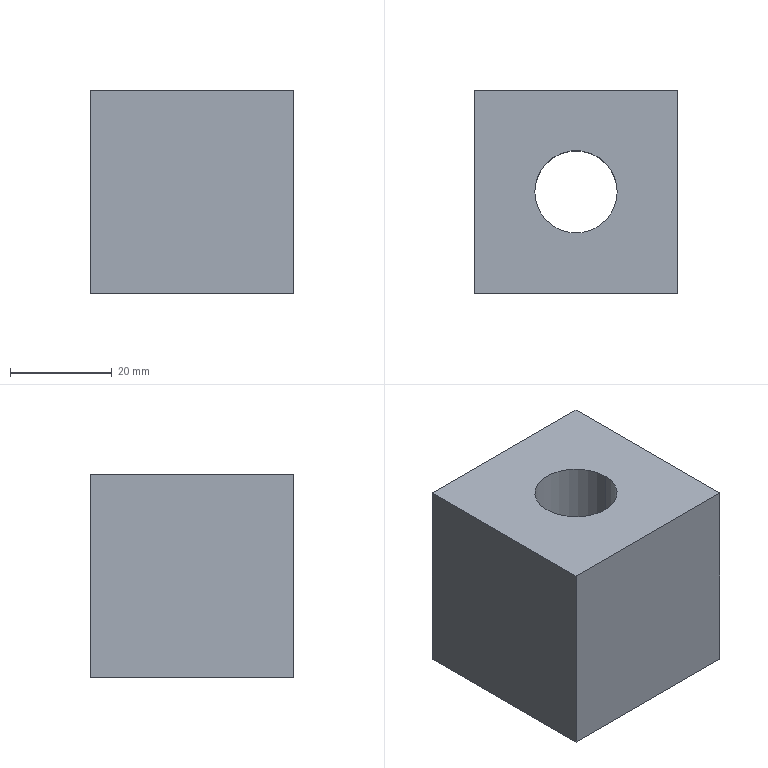Part | SolidWorks | features Extrusion 1, ICE 1 | 1 solid | 8 faces | box 40 x 40 x 40 mm | volume 55755 mm3 | plane 6 | cylinder 2 | commonest cylinder face diameters 16.2 x2
STEP:
#1=CARTESIAN_POINT('',(-8.1,0.,-20.));
#2=VERTEX_POINT('',#1);
#3=CARTESIAN_POINT('',(8.1,0.,-20.));
#4=VERTEX_POINT('',#3);
#5=CARTESIAN_POINT('',(0.,0.,-20.));
#6=DIRECTION('',(0.,0.,1.));
#7=DIRECTION('',(1.,0.,0.));
#8=AXIS2_PLACEMENT_3D('',#5,#6,#7);
#9=CIRCLE('',#8,8.1);
#10=EDGE_CURVE('',#2,#4,#9,.T.);
#11=ORIENTED_EDGE('',*,*,#10,.F.);
#12=CARTESIAN_POINT('',(-8.1,0.,20.));
#13=VERTEX_POINT('',#12);
#14=CARTESIAN_POINT('',(-8.1,0.,-40.));
#15=DIRECTION('',(0.,0.,1.));
#16=VECTOR('',#15,1000.);
#17=LINE('',#14,#16);
#18=EDGE_CURVE('',#2,#13,#17,.T.);
#19=ORIENTED_EDGE('',*,*,#18,.T.);
#20=CARTESIAN_POINT('',(8.1,0.,20.));
#21=VERTEX_POINT('',#20);
#22=CARTESIAN_POINT('',(0.,0.,20.));
#23=DIRECTION('',(0.,0.,1.));
#24=DIRECTION('',(1.,0.,0.));
#25=AXIS2_PLACEMENT_3D('',#22,#23,#24);
#26=CIRCLE('',#25,8.1);
#27=EDGE_CURVE('',#13,#21,#26,.T.);
#28=ORIENTED_EDGE('',*,*,#27,.T.);
#29=CARTESIAN_POINT('',(8.1,0.,-40.));
#30=DIRECTION('',(0.,0.,1.));
#31=VECTOR('',#30,1000.);
#32=LINE('',#29,#31);
#33=EDGE_CURVE('',#4,#21,#32,.T.);
#34=ORIENTED_EDGE('',*,*,#33,.F.);
#35=EDGE_LOOP('',(#11,#19,#28,#34));
#36=FACE_OUTER_BOUND('',#35,.T.);
#37=CARTESIAN_POINT('',(0.,0.,-40.));
#38=DIRECTION('',(0.,0.,1.));
#39=DIRECTION('',(1.,0.,0.));
#40=AXIS2_PLACEMENT_3D('',#37,#38,#39);
#41=CYLINDRICAL_SURFACE('',#40,8.1);
#42=ADVANCED_FACE('',(#36),#41,.F.);
#43=CARTESIAN_POINT('',(-20.,20.,20.));
#44=VERTEX_POINT('',#43);
#45=CARTESIAN_POINT('',(-20.,-20.,20.));
#46=VERTEX_POINT('',#45);
#47=CARTESIAN_POINT('',(-20.,20.,20.));
#48=DIRECTION('',(0.,-1.,0.));
#49=VECTOR('',#48,1000.);
#50=LINE('',#47,#49);
#51=EDGE_CURVE('',#44,#46,#50,.T.);
#52=ORIENTED_EDGE('',*,*,#51,.F.);
#53=CARTESIAN_POINT('',(-20.,20.,-20.));
#54=VERTEX_POINT('',#53);
#55=CARTESIAN_POINT('',(-20.,20.,-20.));
#56=DIRECTION('',(0.,0.,1.));
#57=VECTOR('',#56,1000.);
#58=LINE('',#55,#57);
#59=EDGE_CURVE('',#54,#44,#58,.T.);
#60=ORIENTED_EDGE('',*,*,#59,.F.);
#61=CARTESIAN_POINT('',(-20.,-20.,-20.));
#62=VERTEX_POINT('',#61);
#63=CARTESIAN_POINT('',(-20.,20.,-20.));
#64=DIRECTION('',(0.,-1.,0.));
#65=VECTOR('',#64,1000.);
#66=LINE('',#63,#65);
#67=EDGE_CURVE('',#54,#62,#66,.T.);
#68=ORIENTED_EDGE('',*,*,#67,.T.);
#69=CARTESIAN_POINT('',(-20.,-20.,-20.));
#70=DIRECTION('',(0.,0.,1.));
#71=VECTOR('',#70,1000.);
#72=LINE('',#69,#71);
#73=EDGE_CURVE('',#62,#46,#72,.T.);
#74=ORIENTED_EDGE('',*,*,#73,.T.);
#75=EDGE_LOOP('',(#52,#60,#68,#74));
#76=FACE_OUTER_BOUND('',#75,.T.);
#77=CARTESIAN_POINT('',(-20.,20.,-20.));
#78=DIRECTION('',(-1.,0.,0.));
#79=DIRECTION('',(0.,0.,1.));
#80=AXIS2_PLACEMENT_3D('',#77,#78,#79);
#81=PLANE('',#80);
#82=ADVANCED_FACE('',(#76),#81,.T.);
#83=CARTESIAN_POINT('',(20.,20.,20.));
#84=VERTEX_POINT('',#83);
#85=CARTESIAN_POINT('',(20.,20.,20.));
#86=DIRECTION('',(-1.,0.,0.));
#87=VECTOR('',#86,1000.);
#88=LINE('',#85,#87);
#89=EDGE_CURVE('',#84,#44,#88,.T.);
#90=ORIENTED_EDGE('',*,*,#89,.F.);
#91=CARTESIAN_POINT('',(20.,20.,-20.));
#92=VERTEX_POINT('',#91);
#93=CARTESIAN_POINT('',(20.,20.,-20.));
#94=DIRECTION('',(0.,0.,1.));
#95=VECTOR('',#94,1000.);
#96=LINE('',#93,#95);
#97=EDGE_CURVE('',#92,#84,#96,.T.);
#98=ORIENTED_EDGE('',*,*,#97,.F.);
#99=CARTESIAN_POINT('',(20.,20.,-20.));
#100=DIRECTION('',(-1.,0.,0.));
#101=VECTOR('',#100,1000.);
#102=LINE('',#99,#101);
#103=EDGE_CURVE('',#92,#54,#102,.T.);
#104=ORIENTED_EDGE('',*,*,#103,.T.);
#105=ORIENTED_EDGE('',*,*,#59,.T.);
#106=EDGE_LOOP('',(#90,#98,#104,#105));
#107=FACE_OUTER_BOUND('',#106,.T.);
#108=CARTESIAN_POINT('',(20.,20.,-20.));
#109=DIRECTION('',(0.,1.,0.));
#110=DIRECTION('',(0.,0.,1.));
#111=AXIS2_PLACEMENT_3D('',#108,#109,#110);
#112=PLANE('',#111);
#113=ADVANCED_FACE('',(#107),#112,.T.);
#114=CARTESIAN_POINT('',(20.,-20.,20.));
#115=VERTEX_POINT('',#114);
#116=CARTESIAN_POINT('',(20.,-20.,20.));
#117=DIRECTION('',(0.,1.,0.));
#118=VECTOR('',#117,1000.);
#119=LINE('',#116,#118);
#120=EDGE_CURVE('',#115,#84,#119,.T.);
#121=ORIENTED_EDGE('',*,*,#120,.F.);
#122=CARTESIAN_POINT('',(20.,-20.,-20.));
#123=VERTEX_POINT('',#122);
#124=CARTESIAN_POINT('',(20.,-20.,-20.));
#125=DIRECTION('',(0.,0.,1.));
#126=VECTOR('',#125,1000.);
#127=LINE('',#124,#126);
#128=EDGE_CURVE('',#123,#115,#127,.T.);
#129=ORIENTED_EDGE('',*,*,#128,.F.);
#130=CARTESIAN_POINT('',(20.,-20.,-20.));
#131=DIRECTION('',(0.,1.,0.));
#132=VECTOR('',#131,1000.);
#133=LINE('',#130,#132);
#134=EDGE_CURVE('',#123,#92,#133,.T.);
#135=ORIENTED_EDGE('',*,*,#134,.T.);
#136=ORIENTED_EDGE('',*,*,#97,.T.);
#137=EDGE_LOOP('',(#121,#129,#135,#136));
#138=FACE_OUTER_BOUND('',#137,.T.);
#139=CARTESIAN_POINT('',(20.,-20.,-20.));
#140=DIRECTION('',(1.,0.,0.));
#141=DIRECTION('',(0.,0.,-1.));
#142=AXIS2_PLACEMENT_3D('',#139,#140,#141);
#143=PLANE('',#142);
#144=ADVANCED_FACE('',(#138),#143,.T.);
#145=CARTESIAN_POINT('',(-20.,-20.,20.));
#146=DIRECTION('',(1.,0.,0.));
#147=VECTOR('',#146,1000.);
#148=LINE('',#145,#147);
#149=EDGE_CURVE('',#46,#115,#148,.T.);
#150=ORIENTED_EDGE('',*,*,#149,.F.);
#151=ORIENTED_EDGE('',*,*,#73,.F.);
#152=CARTESIAN_POINT('',(-20.,-20.,-20.));
#153=DIRECTION('',(1.,0.,0.));
#154=VECTOR('',#153,1000.);
#155=LINE('',#152,#154);
#156=EDGE_CURVE('',#62,#123,#155,.T.);
#157=ORIENTED_EDGE('',*,*,#156,.T.);
#158=ORIENTED_EDGE('',*,*,#128,.T.);
#159=EDGE_LOOP('',(#150,#151,#157,#158));
#160=FACE_OUTER_BOUND('',#159,.T.);
#161=CARTESIAN_POINT('',(-20.,-20.,-20.));
#162=DIRECTION('',(0.,-1.,0.));
#163=DIRECTION('',(0.,0.,-1.));
#164=AXIS2_PLACEMENT_3D('',#161,#162,#163);
#165=PLANE('',#164);
#166=ADVANCED_FACE('',(#160),#165,.T.);
#167=CARTESIAN_POINT('',(0.,0.,-20.));
#168=DIRECTION('',(0.,0.,1.));
#169=DIRECTION('',(1.,0.,0.));
#170=AXIS2_PLACEMENT_3D('',#167,#168,#169);
#171=CIRCLE('',#170,8.1);
#172=EDGE_CURVE('',#4,#2,#171,.T.);
#173=ORIENTED_EDGE('',*,*,#172,.T.);
#174=ORIENTED_EDGE('',*,*,#10,.T.);
#175=EDGE_LOOP('',(#173,#174));
#176=FACE_BOUND('',#175,.T.);
#177=ORIENTED_EDGE('',*,*,#67,.F.);
#178=ORIENTED_EDGE('',*,*,#103,.F.);
#179=ORIENTED_EDGE('',*,*,#134,.F.);
#180=ORIENTED_EDGE('',*,*,#156,.F.);
#181=EDGE_LOOP('',(#177,#178,#179,#180));
#182=FACE_OUTER_BOUND('',#181,.T.);
#183=CARTESIAN_POINT('',(0.,0.,-20.));
#184=DIRECTION('',(0.,0.,1.));
#185=DIRECTION('',(1.,0.,0.));
#186=AXIS2_PLACEMENT_3D('',#183,#184,#185);
#187=PLANE('',#186);
#188=ADVANCED_FACE('',(#176,#182),#187,.F.);
#189=CARTESIAN_POINT('',(0.,0.,20.));
#190=DIRECTION('',(0.,0.,1.));
#191=DIRECTION('',(1.,0.,0.));
#192=AXIS2_PLACEMENT_3D('',#189,#190,#191);
#193=CIRCLE('',#192,8.1);
#194=EDGE_CURVE('',#21,#13,#193,.T.);
#195=ORIENTED_EDGE('',*,*,#194,.F.);
#196=ORIENTED_EDGE('',*,*,#27,.F.);
#197=EDGE_LOOP('',(#195,#196));
#198=FACE_BOUND('',#197,.T.);
#199=ORIENTED_EDGE('',*,*,#51,.T.);
#200=ORIENTED_EDGE('',*,*,#149,.T.);
#201=ORIENTED_EDGE('',*,*,#120,.T.);
#202=ORIENTED_EDGE('',*,*,#89,.T.);
#203=EDGE_LOOP('',(#199,#200,#201,#202));
#204=FACE_OUTER_BOUND('',#203,.T.);
#205=CARTESIAN_POINT('',(0.,0.,20.));
#206=DIRECTION('',(0.,0.,1.));
#207=DIRECTION('',(1.,0.,0.));
#208=AXIS2_PLACEMENT_3D('',#205,#206,#207);
#209=PLANE('',#208);
#210=ADVANCED_FACE('',(#198,#204),#209,.T.);
#211=ORIENTED_EDGE('',*,*,#18,.F.);
#212=ORIENTED_EDGE('',*,*,#172,.F.);
#213=ORIENTED_EDGE('',*,*,#33,.T.);
#214=ORIENTED_EDGE('',*,*,#194,.T.);
#215=EDGE_LOOP('',(#211,#212,#213,#214));
#216=FACE_OUTER_BOUND('',#215,.T.);
#217=CARTESIAN_POINT('',(0.,0.,-40.));
#218=DIRECTION('',(0.,0.,1.));
#219=DIRECTION('',(1.,0.,0.));
#220=AXIS2_PLACEMENT_3D('',#217,#218,#219);
#221=CYLINDRICAL_SURFACE('',#220,8.1);
#222=ADVANCED_FACE('',(#216),#221,.F.);
#223=CLOSED_SHELL('',(#42,#82,#113,#144,#166,#188,#210,#222));
#224=MANIFOLD_SOLID_BREP('',#223);
#225=CARTESIAN_POINT('',(0.,0.,0.));
#226=DIRECTION('',(0.,0.,1.));
#227=DIRECTION('',(1.,0.,0.));
#228=AXIS2_PLACEMENT_3D('',#225,#226,#227);
#229=(LENGTH_UNIT()NAMED_UNIT(*)SI_UNIT(.MILLI.,.METRE.));
#230=UNCERTAINTY_MEASURE_WITH_UNIT(LENGTH_MEASURE(0.00001),#229,'','');
#231=(NAMED_UNIT(*)PLANE_ANGLE_UNIT()SI_UNIT($,.RADIAN.));
#232=(NAMED_UNIT(*)SI_UNIT($,.STERADIAN.)SOLID_ANGLE_UNIT());
#233=(GEOMETRIC_REPRESENTATION_CONTEXT(3)GLOBAL_UNCERTAINTY_ASSIGNED_CONTEXT((#230))GLOBAL_UNIT_ASSIGNED_CONTEXT((#229,#231,#232))REPRESENTATION_CONTEXT('',''));
#234=ADVANCED_BREP_SHAPE_REPRESENTATION('',(#224,#228),#233);